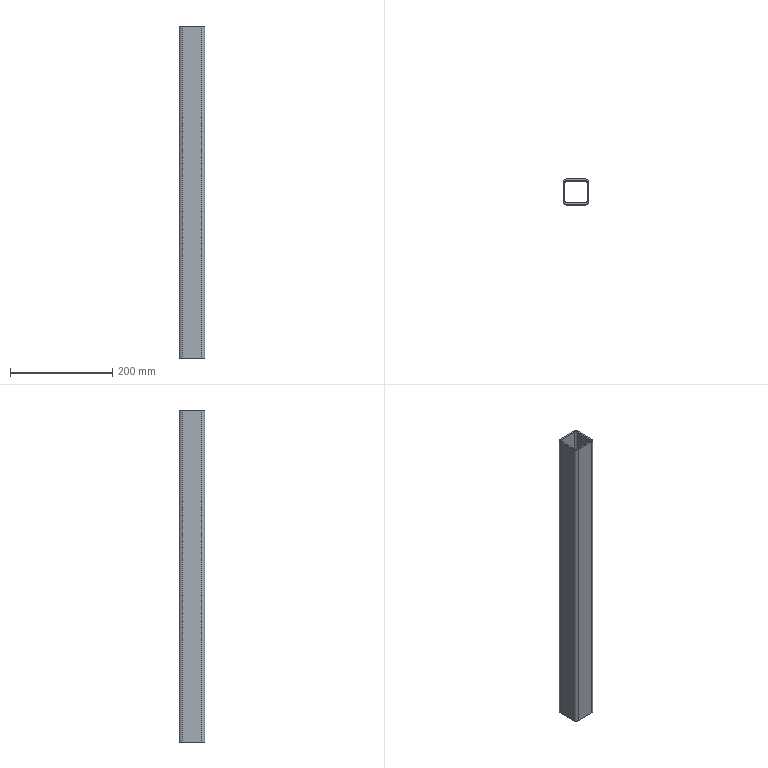Part | STEP file | JIS G 3466 50 x 50 x 3,2 1784904367085 | 1 solid | 18 faces | box 50 x 50 x 650 mm | volume 372235 mm3 | plane 10 | cylinder 8 | commonest cylinder face diameters 6.4 x4 12.8 x4
STEP:
#1=CARTESIAN_POINT('',(25.,-18.6,50.));
#2=VERTEX_POINT('',#1);
#3=CARTESIAN_POINT('',(25.,18.6,50.));
#4=VERTEX_POINT('',#3);
#5=CARTESIAN_POINT('',(25.,9.3,50.));
#6=DIRECTION('',(0.,1.,0.));
#7=VECTOR('',#6,10.);
#8=LINE('',#5,#7);
#9=EDGE_CURVE('',#2,#4,#8,.T.);
#10=ORIENTED_EDGE('',*,*,#9,.F.);
#11=CARTESIAN_POINT('',(18.6,-25.,50.));
#12=VERTEX_POINT('',#11);
#13=CARTESIAN_POINT('',(18.6,-18.6,50.));
#14=DIRECTION('',(0.,0.,1.));
#15=DIRECTION('',(0.,1.,0.));
#16=AXIS2_PLACEMENT_3D('',#13,#14,#15);
#17=CIRCLE('',#16,6.4);
#18=EDGE_CURVE('',#12,#2,#17,.T.);
#19=ORIENTED_EDGE('',*,*,#18,.F.);
#20=CARTESIAN_POINT('',(-18.6,-25.,50.));
#21=VERTEX_POINT('',#20);
#22=CARTESIAN_POINT('',(9.3,-25.,50.));
#23=DIRECTION('',(1.,0.,0.));
#24=VECTOR('',#23,10.);
#25=LINE('',#22,#24);
#26=EDGE_CURVE('',#21,#12,#25,.T.);
#27=ORIENTED_EDGE('',*,*,#26,.F.);
#28=CARTESIAN_POINT('',(-25.,-18.6,50.));
#29=VERTEX_POINT('',#28);
#30=CARTESIAN_POINT('',(-18.6,-18.6,50.));
#31=DIRECTION('',(0.,0.,1.));
#32=DIRECTION('',(1.,0.,0.));
#33=AXIS2_PLACEMENT_3D('',#30,#31,#32);
#34=CIRCLE('',#33,6.4);
#35=EDGE_CURVE('',#29,#21,#34,.T.);
#36=ORIENTED_EDGE('',*,*,#35,.F.);
#37=CARTESIAN_POINT('',(-25.,18.6,50.));
#38=VERTEX_POINT('',#37);
#39=CARTESIAN_POINT('',(-25.,-9.3,50.));
#40=DIRECTION('',(0.,-1.,0.));
#41=VECTOR('',#40,10.);
#42=LINE('',#39,#41);
#43=EDGE_CURVE('',#38,#29,#42,.T.);
#44=ORIENTED_EDGE('',*,*,#43,.F.);
#45=CARTESIAN_POINT('',(-18.6,25.,50.));
#46=VERTEX_POINT('',#45);
#47=CARTESIAN_POINT('',(-18.6,18.6,50.));
#48=DIRECTION('',(0.,0.,1.));
#49=DIRECTION('',(0.,-1.,0.));
#50=AXIS2_PLACEMENT_3D('',#47,#48,#49);
#51=CIRCLE('',#50,6.4);
#52=EDGE_CURVE('',#46,#38,#51,.T.);
#53=ORIENTED_EDGE('',*,*,#52,.F.);
#54=CARTESIAN_POINT('',(18.6,25.,50.));
#55=VERTEX_POINT('',#54);
#56=CARTESIAN_POINT('',(-9.3,25.,50.));
#57=DIRECTION('',(-1.,0.,0.));
#58=VECTOR('',#57,10.);
#59=LINE('',#56,#58);
#60=EDGE_CURVE('',#55,#46,#59,.T.);
#61=ORIENTED_EDGE('',*,*,#60,.F.);
#62=CARTESIAN_POINT('',(18.6,18.6,50.));
#63=DIRECTION('',(0.,0.,1.));
#64=DIRECTION('',(-1.,0.,0.));
#65=AXIS2_PLACEMENT_3D('',#62,#63,#64);
#66=CIRCLE('',#65,6.4);
#67=EDGE_CURVE('',#4,#55,#66,.T.);
#68=ORIENTED_EDGE('',*,*,#67,.F.);
#69=EDGE_LOOP('',(#10,#19,#27,#36,#44,#53,#61,#68));
#70=FACE_OUTER_BOUND('',#69,.T.);
#71=CARTESIAN_POINT('',(18.6,-21.8,50.));
#72=VERTEX_POINT('',#71);
#73=CARTESIAN_POINT('',(-18.6,-21.8,50.));
#74=VERTEX_POINT('',#73);
#75=CARTESIAN_POINT('',(9.3,-21.8,50.));
#76=DIRECTION('',(-1.,0.,0.));
#77=VECTOR('',#76,10.);
#78=LINE('',#75,#77);
#79=EDGE_CURVE('',#72,#74,#78,.T.);
#80=ORIENTED_EDGE('',*,*,#79,.F.);
#81=CARTESIAN_POINT('',(21.8,-18.6,50.));
#82=VERTEX_POINT('',#81);
#83=CARTESIAN_POINT('',(18.6,-18.6,50.));
#84=DIRECTION('',(0.,0.,-1.));
#85=DIRECTION('',(0.,1.,0.));
#86=AXIS2_PLACEMENT_3D('',#83,#84,#85);
#87=CIRCLE('',#86,3.2);
#88=EDGE_CURVE('',#82,#72,#87,.T.);
#89=ORIENTED_EDGE('',*,*,#88,.F.);
#90=CARTESIAN_POINT('',(21.8,18.6,50.));
#91=VERTEX_POINT('',#90);
#92=CARTESIAN_POINT('',(21.8,9.3,50.));
#93=DIRECTION('',(0.,-1.,0.));
#94=VECTOR('',#93,10.);
#95=LINE('',#92,#94);
#96=EDGE_CURVE('',#91,#82,#95,.T.);
#97=ORIENTED_EDGE('',*,*,#96,.F.);
#98=CARTESIAN_POINT('',(18.6,21.8,50.));
#99=VERTEX_POINT('',#98);
#100=CARTESIAN_POINT('',(18.6,18.6,50.));
#101=DIRECTION('',(0.,0.,-1.));
#102=DIRECTION('',(-1.,0.,0.));
#103=AXIS2_PLACEMENT_3D('',#100,#101,#102);
#104=CIRCLE('',#103,3.2);
#105=EDGE_CURVE('',#99,#91,#104,.T.);
#106=ORIENTED_EDGE('',*,*,#105,.F.);
#107=CARTESIAN_POINT('',(-18.6,21.8,50.));
#108=VERTEX_POINT('',#107);
#109=CARTESIAN_POINT('',(-9.3,21.8,50.));
#110=DIRECTION('',(1.,0.,0.));
#111=VECTOR('',#110,10.);
#112=LINE('',#109,#111);
#113=EDGE_CURVE('',#108,#99,#112,.T.);
#114=ORIENTED_EDGE('',*,*,#113,.F.);
#115=CARTESIAN_POINT('',(-21.8,18.6,50.));
#116=VERTEX_POINT('',#115);
#117=CARTESIAN_POINT('',(-18.6,18.6,50.));
#118=DIRECTION('',(0.,0.,-1.));
#119=DIRECTION('',(0.,-1.,0.));
#120=AXIS2_PLACEMENT_3D('',#117,#118,#119);
#121=CIRCLE('',#120,3.2);
#122=EDGE_CURVE('',#116,#108,#121,.T.);
#123=ORIENTED_EDGE('',*,*,#122,.F.);
#124=CARTESIAN_POINT('',(-21.8,-18.6,50.));
#125=VERTEX_POINT('',#124);
#126=CARTESIAN_POINT('',(-21.8,-9.3,50.));
#127=DIRECTION('',(0.,1.,0.));
#128=VECTOR('',#127,10.);
#129=LINE('',#126,#128);
#130=EDGE_CURVE('',#125,#116,#129,.T.);
#131=ORIENTED_EDGE('',*,*,#130,.F.);
#132=CARTESIAN_POINT('',(-18.6,-18.6,50.));
#133=DIRECTION('',(0.,0.,-1.));
#134=DIRECTION('',(1.,0.,0.));
#135=AXIS2_PLACEMENT_3D('',#132,#133,#134);
#136=CIRCLE('',#135,3.2);
#137=EDGE_CURVE('',#74,#125,#136,.T.);
#138=ORIENTED_EDGE('',*,*,#137,.F.);
#139=EDGE_LOOP('',(#80,#89,#97,#106,#114,#123,#131,#138));
#140=FACE_BOUND('',#139,.T.);
#141=CARTESIAN_POINT('',(0.,0.,50.));
#142=DIRECTION('',(0.,0.,1.));
#143=DIRECTION('',(1.,0.,0.));
#144=AXIS2_PLACEMENT_3D('',#141,#142,#143);
#145=PLANE('',#144);
#146=ADVANCED_FACE('',(#70,#140),#145,.F.);
#147=ORIENTED_EDGE('',*,*,#113,.T.);
#148=CARTESIAN_POINT('',(18.6,21.8,700.));
#149=VERTEX_POINT('',#148);
#150=CARTESIAN_POINT('',(18.6,21.8,0.));
#151=DIRECTION('',(0.,0.,1.));
#152=VECTOR('',#151,10.);
#153=LINE('',#150,#152);
#154=EDGE_CURVE('',#99,#149,#153,.T.);
#155=ORIENTED_EDGE('',*,*,#154,.T.);
#156=CARTESIAN_POINT('',(-18.6,21.8,700.));
#157=VERTEX_POINT('',#156);
#158=CARTESIAN_POINT('',(-9.3,21.8,700.));
#159=DIRECTION('',(-1.,0.,0.));
#160=VECTOR('',#159,10.);
#161=LINE('',#158,#160);
#162=EDGE_CURVE('',#149,#157,#161,.T.);
#163=ORIENTED_EDGE('',*,*,#162,.T.);
#164=CARTESIAN_POINT('',(-18.6,21.8,0.));
#165=DIRECTION('',(0.,0.,1.));
#166=VECTOR('',#165,10.);
#167=LINE('',#164,#166);
#168=EDGE_CURVE('',#108,#157,#167,.T.);
#169=ORIENTED_EDGE('',*,*,#168,.F.);
#170=EDGE_LOOP('',(#147,#155,#163,#169));
#171=FACE_OUTER_BOUND('',#170,.T.);
#172=CARTESIAN_POINT('',(-18.6,21.8,0.));
#173=DIRECTION('',(0.,1.,0.));
#174=DIRECTION('',(0.,0.,1.));
#175=AXIS2_PLACEMENT_3D('',#172,#173,#174);
#176=PLANE('',#175);
#177=ADVANCED_FACE('',(#171),#176,.F.);
#178=ORIENTED_EDGE('',*,*,#105,.T.);
#179=CARTESIAN_POINT('',(21.8,18.6,700.));
#180=VERTEX_POINT('',#179);
#181=CARTESIAN_POINT('',(21.8,18.6,0.));
#182=DIRECTION('',(0.,0.,1.));
#183=VECTOR('',#182,10.);
#184=LINE('',#181,#183);
#185=EDGE_CURVE('',#91,#180,#184,.T.);
#186=ORIENTED_EDGE('',*,*,#185,.T.);
#187=CARTESIAN_POINT('',(18.6,18.6,700.));
#188=DIRECTION('',(0.,0.,1.));
#189=DIRECTION('',(-1.,0.,0.));
#190=AXIS2_PLACEMENT_3D('',#187,#188,#189);
#191=CIRCLE('',#190,3.2);
#192=EDGE_CURVE('',#180,#149,#191,.T.);
#193=ORIENTED_EDGE('',*,*,#192,.T.);
#194=ORIENTED_EDGE('',*,*,#154,.F.);
#195=EDGE_LOOP('',(#178,#186,#193,#194));
#196=FACE_OUTER_BOUND('',#195,.T.);
#197=CARTESIAN_POINT('',(18.6,18.6,0.));
#198=DIRECTION('',(0.,0.,1.));
#199=DIRECTION('',(-1.,0.,0.));
#200=AXIS2_PLACEMENT_3D('',#197,#198,#199);
#201=CYLINDRICAL_SURFACE('',#200,3.2);
#202=ADVANCED_FACE('',(#196),#201,.F.);
#203=ORIENTED_EDGE('',*,*,#96,.T.);
#204=CARTESIAN_POINT('',(21.8,-18.6,700.));
#205=VERTEX_POINT('',#204);
#206=CARTESIAN_POINT('',(21.8,-18.6,0.));
#207=DIRECTION('',(0.,0.,1.));
#208=VECTOR('',#207,10.);
#209=LINE('',#206,#208);
#210=EDGE_CURVE('',#82,#205,#209,.T.);
#211=ORIENTED_EDGE('',*,*,#210,.T.);
#212=CARTESIAN_POINT('',(21.8,9.3,700.));
#213=DIRECTION('',(0.,1.,0.));
#214=VECTOR('',#213,10.);
#215=LINE('',#212,#214);
#216=EDGE_CURVE('',#205,#180,#215,.T.);
#217=ORIENTED_EDGE('',*,*,#216,.T.);
#218=ORIENTED_EDGE('',*,*,#185,.F.);
#219=EDGE_LOOP('',(#203,#211,#217,#218));
#220=FACE_OUTER_BOUND('',#219,.T.);
#221=CARTESIAN_POINT('',(21.8,18.6,0.));
#222=DIRECTION('',(1.,0.,0.));
#223=DIRECTION('',(0.,0.,-1.));
#224=AXIS2_PLACEMENT_3D('',#221,#222,#223);
#225=PLANE('',#224);
#226=ADVANCED_FACE('',(#220),#225,.F.);
#227=ORIENTED_EDGE('',*,*,#88,.T.);
#228=CARTESIAN_POINT('',(18.6,-21.8,700.));
#229=VERTEX_POINT('',#228);
#230=CARTESIAN_POINT('',(18.6,-21.8,0.));
#231=DIRECTION('',(0.,0.,1.));
#232=VECTOR('',#231,10.);
#233=LINE('',#230,#232);
#234=EDGE_CURVE('',#72,#229,#233,.T.);
#235=ORIENTED_EDGE('',*,*,#234,.T.);
#236=CARTESIAN_POINT('',(18.6,-18.6,700.));
#237=DIRECTION('',(0.,0.,1.));
#238=DIRECTION('',(0.,1.,0.));
#239=AXIS2_PLACEMENT_3D('',#236,#237,#238);
#240=CIRCLE('',#239,3.2);
#241=EDGE_CURVE('',#229,#205,#240,.T.);
#242=ORIENTED_EDGE('',*,*,#241,.T.);
#243=ORIENTED_EDGE('',*,*,#210,.F.);
#244=EDGE_LOOP('',(#227,#235,#242,#243));
#245=FACE_OUTER_BOUND('',#244,.T.);
#246=CARTESIAN_POINT('',(18.6,-18.6,0.));
#247=DIRECTION('',(0.,0.,1.));
#248=DIRECTION('',(0.,1.,0.));
#249=AXIS2_PLACEMENT_3D('',#246,#247,#248);
#250=CYLINDRICAL_SURFACE('',#249,3.2);
#251=ADVANCED_FACE('',(#245),#250,.F.);
#252=ORIENTED_EDGE('',*,*,#43,.T.);
#253=CARTESIAN_POINT('',(-25.,-18.6,700.));
#254=VERTEX_POINT('',#253);
#255=CARTESIAN_POINT('',(-25.,-18.6,0.));
#256=DIRECTION('',(0.,0.,1.));
#257=VECTOR('',#256,10.);
#258=LINE('',#255,#257);
#259=EDGE_CURVE('',#29,#254,#258,.T.);
#260=ORIENTED_EDGE('',*,*,#259,.T.);
#261=CARTESIAN_POINT('',(-25.,18.6,700.));
#262=VERTEX_POINT('',#261);
#263=CARTESIAN_POINT('',(-25.,-9.3,700.));
#264=DIRECTION('',(0.,1.,0.));
#265=VECTOR('',#264,10.);
#266=LINE('',#263,#265);
#267=EDGE_CURVE('',#254,#262,#266,.T.);
#268=ORIENTED_EDGE('',*,*,#267,.T.);
#269=CARTESIAN_POINT('',(-25.,18.6,0.));
#270=DIRECTION('',(0.,0.,1.));
#271=VECTOR('',#270,10.);
#272=LINE('',#269,#271);
#273=EDGE_CURVE('',#38,#262,#272,.T.);
#274=ORIENTED_EDGE('',*,*,#273,.F.);
#275=EDGE_LOOP('',(#252,#260,#268,#274));
#276=FACE_OUTER_BOUND('',#275,.T.);
#277=CARTESIAN_POINT('',(-25.,-18.6,0.));
#278=DIRECTION('',(-1.,0.,0.));
#279=DIRECTION('',(0.,0.,1.));
#280=AXIS2_PLACEMENT_3D('',#277,#278,#279);
#281=PLANE('',#280);
#282=ADVANCED_FACE('',(#276),#281,.T.);
#283=ORIENTED_EDGE('',*,*,#35,.T.);
#284=CARTESIAN_POINT('',(-18.6,-25.,700.));
#285=VERTEX_POINT('',#284);
#286=CARTESIAN_POINT('',(-18.6,-25.,0.));
#287=DIRECTION('',(0.,0.,1.));
#288=VECTOR('',#287,10.);
#289=LINE('',#286,#288);
#290=EDGE_CURVE('',#21,#285,#289,.T.);
#291=ORIENTED_EDGE('',*,*,#290,.T.);
#292=CARTESIAN_POINT('',(-18.6,-18.6,700.));
#293=DIRECTION('',(0.,0.,-1.));
#294=DIRECTION('',(1.,0.,0.));
#295=AXIS2_PLACEMENT_3D('',#292,#293,#294);
#296=CIRCLE('',#295,6.4);
#297=EDGE_CURVE('',#285,#254,#296,.T.);
#298=ORIENTED_EDGE('',*,*,#297,.T.);
#299=ORIENTED_EDGE('',*,*,#259,.F.);
#300=EDGE_LOOP('',(#283,#291,#298,#299));
#301=FACE_OUTER_BOUND('',#300,.T.);
#302=CARTESIAN_POINT('',(-18.6,-18.6,0.));
#303=DIRECTION('',(0.,0.,1.));
#304=DIRECTION('',(1.,0.,0.));
#305=AXIS2_PLACEMENT_3D('',#302,#303,#304);
#306=CYLINDRICAL_SURFACE('',#305,6.4);
#307=ADVANCED_FACE('',(#301),#306,.T.);
#308=ORIENTED_EDGE('',*,*,#26,.T.);
#309=CARTESIAN_POINT('',(18.6,-25.,700.));
#310=VERTEX_POINT('',#309);
#311=CARTESIAN_POINT('',(18.6,-25.,0.));
#312=DIRECTION('',(0.,0.,1.));
#313=VECTOR('',#312,10.);
#314=LINE('',#311,#313);
#315=EDGE_CURVE('',#12,#310,#314,.T.);
#316=ORIENTED_EDGE('',*,*,#315,.T.);
#317=CARTESIAN_POINT('',(9.3,-25.,700.));
#318=DIRECTION('',(-1.,0.,0.));
#319=VECTOR('',#318,10.);
#320=LINE('',#317,#319);
#321=EDGE_CURVE('',#310,#285,#320,.T.);
#322=ORIENTED_EDGE('',*,*,#321,.T.);
#323=ORIENTED_EDGE('',*,*,#290,.F.);
#324=EDGE_LOOP('',(#308,#316,#322,#323));
#325=FACE_OUTER_BOUND('',#324,.T.);
#326=CARTESIAN_POINT('',(18.6,-25.,0.));
#327=DIRECTION('',(0.,-1.,0.));
#328=DIRECTION('',(0.,0.,-1.));
#329=AXIS2_PLACEMENT_3D('',#326,#327,#328);
#330=PLANE('',#329);
#331=ADVANCED_FACE('',(#325),#330,.T.);
#332=ORIENTED_EDGE('',*,*,#18,.T.);
#333=CARTESIAN_POINT('',(25.,-18.6,700.));
#334=VERTEX_POINT('',#333);
#335=CARTESIAN_POINT('',(25.,-18.6,0.));
#336=DIRECTION('',(0.,0.,1.));
#337=VECTOR('',#336,10.);
#338=LINE('',#335,#337);
#339=EDGE_CURVE('',#2,#334,#338,.T.);
#340=ORIENTED_EDGE('',*,*,#339,.T.);
#341=CARTESIAN_POINT('',(18.6,-18.6,700.));
#342=DIRECTION('',(0.,0.,-1.));
#343=DIRECTION('',(0.,1.,0.));
#344=AXIS2_PLACEMENT_3D('',#341,#342,#343);
#345=CIRCLE('',#344,6.4);
#346=EDGE_CURVE('',#334,#310,#345,.T.);
#347=ORIENTED_EDGE('',*,*,#346,.T.);
#348=ORIENTED_EDGE('',*,*,#315,.F.);
#349=EDGE_LOOP('',(#332,#340,#347,#348));
#350=FACE_OUTER_BOUND('',#349,.T.);
#351=CARTESIAN_POINT('',(18.6,-18.6,0.));
#352=DIRECTION('',(0.,0.,1.));
#353=DIRECTION('',(0.,1.,0.));
#354=AXIS2_PLACEMENT_3D('',#351,#352,#353);
#355=CYLINDRICAL_SURFACE('',#354,6.4);
#356=ADVANCED_FACE('',(#350),#355,.T.);
#357=ORIENTED_EDGE('',*,*,#79,.T.);
#358=CARTESIAN_POINT('',(-18.6,-21.8,700.));
#359=VERTEX_POINT('',#358);
#360=CARTESIAN_POINT('',(-18.6,-21.8,0.));
#361=DIRECTION('',(0.,0.,1.));
#362=VECTOR('',#361,10.);
#363=LINE('',#360,#362);
#364=EDGE_CURVE('',#74,#359,#363,.T.);
#365=ORIENTED_EDGE('',*,*,#364,.T.);
#366=CARTESIAN_POINT('',(9.3,-21.8,700.));
#367=DIRECTION('',(1.,0.,0.));
#368=VECTOR('',#367,10.);
#369=LINE('',#366,#368);
#370=EDGE_CURVE('',#359,#229,#369,.T.);
#371=ORIENTED_EDGE('',*,*,#370,.T.);
#372=ORIENTED_EDGE('',*,*,#234,.F.);
#373=EDGE_LOOP('',(#357,#365,#371,#372));
#374=FACE_OUTER_BOUND('',#373,.T.);
#375=CARTESIAN_POINT('',(18.6,-21.8,0.));
#376=DIRECTION('',(0.,-1.,0.));
#377=DIRECTION('',(0.,0.,-1.));
#378=AXIS2_PLACEMENT_3D('',#375,#376,#377);
#379=PLANE('',#378);
#380=ADVANCED_FACE('',(#374),#379,.F.);
#381=ORIENTED_EDGE('',*,*,#9,.T.);
#382=CARTESIAN_POINT('',(25.,18.6,700.));
#383=VERTEX_POINT('',#382);
#384=CARTESIAN_POINT('',(25.,18.6,0.));
#385=DIRECTION('',(0.,0.,1.));
#386=VECTOR('',#385,10.);
#387=LINE('',#384,#386);
#388=EDGE_CURVE('',#4,#383,#387,.T.);
#389=ORIENTED_EDGE('',*,*,#388,.T.);
#390=CARTESIAN_POINT('',(25.,9.3,700.));
#391=DIRECTION('',(0.,-1.,0.));
#392=VECTOR('',#391,10.);
#393=LINE('',#390,#392);
#394=EDGE_CURVE('',#383,#334,#393,.T.);
#395=ORIENTED_EDGE('',*,*,#394,.T.);
#396=ORIENTED_EDGE('',*,*,#339,.F.);
#397=EDGE_LOOP('',(#381,#389,#395,#396));
#398=FACE_OUTER_BOUND('',#397,.T.);
#399=CARTESIAN_POINT('',(25.,18.6,0.));
#400=DIRECTION('',(1.,0.,0.));
#401=DIRECTION('',(0.,0.,-1.));
#402=AXIS2_PLACEMENT_3D('',#399,#400,#401);
#403=PLANE('',#402);
#404=ADVANCED_FACE('',(#398),#403,.T.);
#405=ORIENTED_EDGE('',*,*,#137,.T.);
#406=CARTESIAN_POINT('',(-21.8,-18.6,700.));
#407=VERTEX_POINT('',#406);
#408=CARTESIAN_POINT('',(-21.8,-18.6,0.));
#409=DIRECTION('',(0.,0.,1.));
#410=VECTOR('',#409,10.);
#411=LINE('',#408,#410);
#412=EDGE_CURVE('',#125,#407,#411,.T.);
#413=ORIENTED_EDGE('',*,*,#412,.T.);
#414=CARTESIAN_POINT('',(-18.6,-18.6,700.));
#415=DIRECTION('',(0.,0.,1.));
#416=DIRECTION('',(1.,0.,0.));
#417=AXIS2_PLACEMENT_3D('',#414,#415,#416);
#418=CIRCLE('',#417,3.2);
#419=EDGE_CURVE('',#407,#359,#418,.T.);
#420=ORIENTED_EDGE('',*,*,#419,.T.);
#421=ORIENTED_EDGE('',*,*,#364,.F.);
#422=EDGE_LOOP('',(#405,#413,#420,#421));
#423=FACE_OUTER_BOUND('',#422,.T.);
#424=CARTESIAN_POINT('',(-18.6,-18.6,0.));
#425=DIRECTION('',(0.,0.,1.));
#426=DIRECTION('',(1.,0.,0.));
#427=AXIS2_PLACEMENT_3D('',#424,#425,#426);
#428=CYLINDRICAL_SURFACE('',#427,3.2);
#429=ADVANCED_FACE('',(#423),#428,.F.);
#430=ORIENTED_EDGE('',*,*,#130,.T.);
#431=CARTESIAN_POINT('',(-21.8,18.6,700.));
#432=VERTEX_POINT('',#431);
#433=CARTESIAN_POINT('',(-21.8,18.6,0.));
#434=DIRECTION('',(0.,0.,1.));
#435=VECTOR('',#434,10.);
#436=LINE('',#433,#435);
#437=EDGE_CURVE('',#116,#432,#436,.T.);
#438=ORIENTED_EDGE('',*,*,#437,.T.);
#439=CARTESIAN_POINT('',(-21.8,-9.3,700.));
#440=DIRECTION('',(0.,-1.,0.));
#441=VECTOR('',#440,10.);
#442=LINE('',#439,#441);
#443=EDGE_CURVE('',#432,#407,#442,.T.);
#444=ORIENTED_EDGE('',*,*,#443,.T.);
#445=ORIENTED_EDGE('',*,*,#412,.F.);
#446=EDGE_LOOP('',(#430,#438,#444,#445));
#447=FACE_OUTER_BOUND('',#446,.T.);
#448=CARTESIAN_POINT('',(-21.8,-18.6,0.));
#449=DIRECTION('',(-1.,0.,0.));
#450=DIRECTION('',(0.,0.,1.));
#451=AXIS2_PLACEMENT_3D('',#448,#449,#450);
#452=PLANE('',#451);
#453=ADVANCED_FACE('',(#447),#452,.F.);
#454=ORIENTED_EDGE('',*,*,#122,.T.);
#455=ORIENTED_EDGE('',*,*,#168,.T.);
#456=CARTESIAN_POINT('',(-18.6,18.6,700.));
#457=DIRECTION('',(0.,0.,1.));
#458=DIRECTION('',(0.,-1.,0.));
#459=AXIS2_PLACEMENT_3D('',#456,#457,#458);
#460=CIRCLE('',#459,3.2);
#461=EDGE_CURVE('',#157,#432,#460,.T.);
#462=ORIENTED_EDGE('',*,*,#461,.T.);
#463=ORIENTED_EDGE('',*,*,#437,.F.);
#464=EDGE_LOOP('',(#454,#455,#462,#463));
#465=FACE_OUTER_BOUND('',#464,.T.);
#466=CARTESIAN_POINT('',(-18.6,18.6,0.));
#467=DIRECTION('',(0.,0.,1.));
#468=DIRECTION('',(0.,-1.,0.));
#469=AXIS2_PLACEMENT_3D('',#466,#467,#468);
#470=CYLINDRICAL_SURFACE('',#469,3.2);
#471=ADVANCED_FACE('',(#465),#470,.F.);
#472=ORIENTED_EDGE('',*,*,#52,.T.);
#473=ORIENTED_EDGE('',*,*,#273,.T.);
#474=CARTESIAN_POINT('',(-18.6,25.,700.));
#475=VERTEX_POINT('',#474);
#476=CARTESIAN_POINT('',(-18.6,18.6,700.));
#477=DIRECTION('',(0.,0.,-1.));
#478=DIRECTION('',(0.,-1.,0.));
#479=AXIS2_PLACEMENT_3D('',#476,#477,#478);
#480=CIRCLE('',#479,6.4);
#481=EDGE_CURVE('',#262,#475,#480,.T.);
#482=ORIENTED_EDGE('',*,*,#481,.T.);
#483=CARTESIAN_POINT('',(-18.6,25.,0.));
#484=DIRECTION('',(0.,0.,1.));
#485=VECTOR('',#484,10.);
#486=LINE('',#483,#485);
#487=EDGE_CURVE('',#46,#475,#486,.T.);
#488=ORIENTED_EDGE('',*,*,#487,.F.);
#489=EDGE_LOOP('',(#472,#473,#482,#488));
#490=FACE_OUTER_BOUND('',#489,.T.);
#491=CARTESIAN_POINT('',(-18.6,18.6,0.));
#492=DIRECTION('',(0.,0.,1.));
#493=DIRECTION('',(0.,-1.,0.));
#494=AXIS2_PLACEMENT_3D('',#491,#492,#493);
#495=CYLINDRICAL_SURFACE('',#494,6.4);
#496=ADVANCED_FACE('',(#490),#495,.T.);
#497=ORIENTED_EDGE('',*,*,#60,.T.);
#498=ORIENTED_EDGE('',*,*,#487,.T.);
#499=CARTESIAN_POINT('',(18.6,25.,700.));
#500=VERTEX_POINT('',#499);
#501=CARTESIAN_POINT('',(-9.3,25.,700.));
#502=DIRECTION('',(1.,0.,0.));
#503=VECTOR('',#502,10.);
#504=LINE('',#501,#503);
#505=EDGE_CURVE('',#475,#500,#504,.T.);
#506=ORIENTED_EDGE('',*,*,#505,.T.);
#507=CARTESIAN_POINT('',(18.6,25.,0.));
#508=DIRECTION('',(0.,0.,1.));
#509=VECTOR('',#508,10.);
#510=LINE('',#507,#509);
#511=EDGE_CURVE('',#55,#500,#510,.T.);
#512=ORIENTED_EDGE('',*,*,#511,.F.);
#513=EDGE_LOOP('',(#497,#498,#506,#512));
#514=FACE_OUTER_BOUND('',#513,.T.);
#515=CARTESIAN_POINT('',(-18.6,25.,0.));
#516=DIRECTION('',(0.,1.,0.));
#517=DIRECTION('',(0.,0.,1.));
#518=AXIS2_PLACEMENT_3D('',#515,#516,#517);
#519=PLANE('',#518);
#520=ADVANCED_FACE('',(#514),#519,.T.);
#521=ORIENTED_EDGE('',*,*,#67,.T.);
#522=ORIENTED_EDGE('',*,*,#511,.T.);
#523=CARTESIAN_POINT('',(18.6,18.6,700.));
#524=DIRECTION('',(0.,0.,-1.));
#525=DIRECTION('',(-1.,0.,0.));
#526=AXIS2_PLACEMENT_3D('',#523,#524,#525);
#527=CIRCLE('',#526,6.4);
#528=EDGE_CURVE('',#500,#383,#527,.T.);
#529=ORIENTED_EDGE('',*,*,#528,.T.);
#530=ORIENTED_EDGE('',*,*,#388,.F.);
#531=EDGE_LOOP('',(#521,#522,#529,#530));
#532=FACE_OUTER_BOUND('',#531,.T.);
#533=CARTESIAN_POINT('',(18.6,18.6,0.));
#534=DIRECTION('',(0.,0.,1.));
#535=DIRECTION('',(-1.,0.,0.));
#536=AXIS2_PLACEMENT_3D('',#533,#534,#535);
#537=CYLINDRICAL_SURFACE('',#536,6.4);
#538=ADVANCED_FACE('',(#532),#537,.T.);
#539=ORIENTED_EDGE('',*,*,#267,.F.);
#540=ORIENTED_EDGE('',*,*,#297,.F.);
#541=ORIENTED_EDGE('',*,*,#321,.F.);
#542=ORIENTED_EDGE('',*,*,#346,.F.);
#543=ORIENTED_EDGE('',*,*,#394,.F.);
#544=ORIENTED_EDGE('',*,*,#528,.F.);
#545=ORIENTED_EDGE('',*,*,#505,.F.);
#546=ORIENTED_EDGE('',*,*,#481,.F.);
#547=EDGE_LOOP('',(#539,#540,#541,#542,#543,#544,#545,#546));
#548=FACE_OUTER_BOUND('',#547,.T.);
#549=ORIENTED_EDGE('',*,*,#162,.F.);
#550=ORIENTED_EDGE('',*,*,#192,.F.);
#551=ORIENTED_EDGE('',*,*,#216,.F.);
#552=ORIENTED_EDGE('',*,*,#241,.F.);
#553=ORIENTED_EDGE('',*,*,#370,.F.);
#554=ORIENTED_EDGE('',*,*,#419,.F.);
#555=ORIENTED_EDGE('',*,*,#443,.F.);
#556=ORIENTED_EDGE('',*,*,#461,.F.);
#557=EDGE_LOOP('',(#549,#550,#551,#552,#553,#554,#555,#556));
#558=FACE_BOUND('',#557,.T.);
#559=CARTESIAN_POINT('',(0.,0.,700.));
#560=DIRECTION('',(0.,0.,1.));
#561=DIRECTION('',(1.,0.,0.));
#562=AXIS2_PLACEMENT_3D('',#559,#560,#561);
#563=PLANE('',#562);
#564=ADVANCED_FACE('',(#548,#558),#563,.T.);
#565=CLOSED_SHELL('',(#146,#177,#202,#226,#251,#282,#307,#331,#356,#380,#404,#429,#453,#471,#496,#520,#538,#564));
#566=MANIFOLD_SOLID_BREP('',#565);
#567=(LENGTH_UNIT()NAMED_UNIT(*)SI_UNIT(.MILLI.,.METRE.));
#568=UNCERTAINTY_MEASURE_WITH_UNIT(LENGTH_MEASURE(0.01),#567,'','');
#569=(NAMED_UNIT(*)PLANE_ANGLE_UNIT()SI_UNIT($,.RADIAN.));
#570=(NAMED_UNIT(*)SI_UNIT($,.STERADIAN.)SOLID_ANGLE_UNIT());
#571=(GEOMETRIC_REPRESENTATION_CONTEXT(3)GLOBAL_UNCERTAINTY_ASSIGNED_CONTEXT((#568))GLOBAL_UNIT_ASSIGNED_CONTEXT((#567,#569,#570))REPRESENTATION_CONTEXT('',''));
#572=ADVANCED_BREP_SHAPE_REPRESENTATION('',(#566),#571);